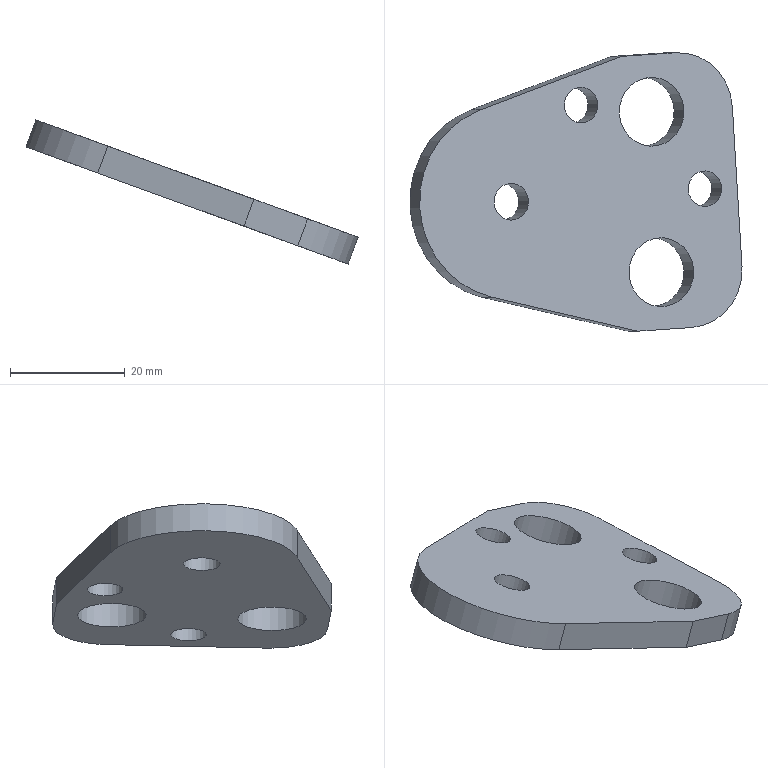Part | NX | features solid 2 | 1 solid | 15 faces | box 57.932 x 48.562 x 25.162 mm | volume 9858 mm3 | cylinder 8 | plane 7 | commonest cylinder face diameters 6.2 x2 12 x2 20 x2 6.4 x1 34 x1
STEP:
#1=CARTESIAN_POINT('',(737.004,494.915,31.011));
#2=VERTEX_POINT('',#1);
#3=CARTESIAN_POINT('',(746.983,485.575,27.379));
#4=VERTEX_POINT('',#3);
#5=CARTESIAN_POINT('',(737.605,484.935,30.792));
#6=DIRECTION('',(-0.342,0.,-0.9397));
#7=DIRECTION('',(0.9378,0.06398,-0.3413));
#8=AXIS2_PLACEMENT_3D('',#5,#6,#7);
#9=CIRCLE('',#8,10.);
#10=EDGE_CURVE('',#2,#4,#9,.T.);
#11=ORIENTED_EDGE('',*,*,#10,.F.);
#12=CARTESIAN_POINT('',(738.714,494.915,35.71));
#13=VERTEX_POINT('',#12);
#14=CARTESIAN_POINT('',(738.714,494.915,35.71));
#15=DIRECTION('',(-0.342,0.,-0.9397));
#16=VECTOR('',#15,1000.);
#17=LINE('',#14,#16);
#18=EDGE_CURVE('',#13,#2,#17,.T.);
#19=ORIENTED_EDGE('',*,*,#18,.F.);
#20=CARTESIAN_POINT('',(748.693,485.575,32.078));
#21=VERTEX_POINT('',#20);
#22=CARTESIAN_POINT('',(739.315,484.935,35.491));
#23=DIRECTION('',(-0.342,0.,-0.9397));
#24=DIRECTION('',(0.9378,0.06398,-0.3413));
#25=AXIS2_PLACEMENT_3D('',#22,#23,#24);
#26=CIRCLE('',#25,10.);
#27=EDGE_CURVE('',#13,#21,#26,.T.);
#28=ORIENTED_EDGE('',*,*,#27,.T.);
#29=CARTESIAN_POINT('',(748.693,485.575,32.078));
#30=DIRECTION('',(-0.342,0.,-0.9397));
#31=VECTOR('',#30,1000.);
#32=LINE('',#29,#31);
#33=EDGE_CURVE('',#21,#4,#32,.T.);
#34=ORIENTED_EDGE('',*,*,#33,.T.);
#35=EDGE_LOOP('',(#11,#19,#28,#34));
#36=FACE_BOUND('',#35,.T.);
#37=CARTESIAN_POINT('',(739.315,484.935,35.491));
#38=DIRECTION('',(-0.342,0.,-0.9397));
#39=DIRECTION('',(0.9378,0.06398,-0.3413));
#40=AXIS2_PLACEMENT_3D('',#37,#38,#39);
#41=CYLINDRICAL_SURFACE('',#40,10.);
#42=ADVANCED_FACE('',(#36),#41,.T.);
#43=CARTESIAN_POINT('',(748.666,457.633,26.766));
#44=VERTEX_POINT('',#43);
#45=CARTESIAN_POINT('',(748.666,457.633,26.766));
#46=DIRECTION('',(-0.06013,0.998,0.02188));
#47=VECTOR('',#46,1000.);
#48=LINE('',#45,#47);
#49=EDGE_CURVE('',#44,#4,#48,.T.);
#50=ORIENTED_EDGE('',*,*,#49,.T.);
#51=ORIENTED_EDGE('',*,*,#33,.F.);
#52=CARTESIAN_POINT('',(750.376,457.633,31.465));
#53=VERTEX_POINT('',#52);
#54=CARTESIAN_POINT('',(750.376,457.633,31.465));
#55=DIRECTION('',(-0.06013,0.998,0.02188));
#56=VECTOR('',#55,1000.);
#57=LINE('',#54,#56);
#58=EDGE_CURVE('',#53,#21,#57,.T.);
#59=ORIENTED_EDGE('',*,*,#58,.F.);
#60=CARTESIAN_POINT('',(750.376,457.633,31.465));
#61=DIRECTION('',(-0.342,0.,-0.9397));
#62=VECTOR('',#61,1000.);
#63=LINE('',#60,#62);
#64=EDGE_CURVE('',#53,#44,#63,.T.);
#65=ORIENTED_EDGE('',*,*,#64,.T.);
#66=EDGE_LOOP('',(#50,#51,#59,#65));
#67=FACE_BOUND('',#66,.T.);
#68=CARTESIAN_POINT('',(750.376,457.633,31.465));
#69=DIRECTION('',(-0.9378,-0.06398,0.3413));
#70=DIRECTION('',(0.06013,-0.998,-0.02188));
#71=AXIS2_PLACEMENT_3D('',#68,#69,#70);
#72=PLANE('',#71);
#73=ADVANCED_FACE('',(#67),#72,.F.);
#74=CARTESIAN_POINT('',(739.89,447.013,29.961));
#75=VERTEX_POINT('',#74);
#76=CARTESIAN_POINT('',(739.289,456.993,30.18));
#77=DIRECTION('',(-0.342,0.,-0.9397));
#78=DIRECTION('',(0.9378,0.06398,-0.3413));
#79=AXIS2_PLACEMENT_3D('',#76,#77,#78);
#80=CIRCLE('',#79,10.);
#81=EDGE_CURVE('',#44,#75,#80,.T.);
#82=ORIENTED_EDGE('',*,*,#81,.F.);
#83=ORIENTED_EDGE('',*,*,#64,.F.);
#84=CARTESIAN_POINT('',(741.6,447.013,34.659));
#85=VERTEX_POINT('',#84);
#86=CARTESIAN_POINT('',(740.999,456.993,34.878));
#87=DIRECTION('',(-0.342,0.,-0.9397));
#88=DIRECTION('',(0.9378,0.06398,-0.3413));
#89=AXIS2_PLACEMENT_3D('',#86,#87,#88);
#90=CIRCLE('',#89,10.);
#91=EDGE_CURVE('',#53,#85,#90,.T.);
#92=ORIENTED_EDGE('',*,*,#91,.T.);
#93=CARTESIAN_POINT('',(741.6,447.013,34.659));
#94=DIRECTION('',(-0.342,0.,-0.9397));
#95=VECTOR('',#94,1000.);
#96=LINE('',#93,#95);
#97=EDGE_CURVE('',#85,#75,#96,.T.);
#98=ORIENTED_EDGE('',*,*,#97,.T.);
#99=EDGE_LOOP('',(#82,#83,#92,#98));
#100=FACE_BOUND('',#99,.T.);
#101=CARTESIAN_POINT('',(740.999,456.993,34.878));
#102=DIRECTION('',(-0.342,0.,-0.9397));
#103=DIRECTION('',(0.9378,0.06398,-0.3413));
#104=AXIS2_PLACEMENT_3D('',#101,#102,#103);
#105=CYLINDRICAL_SURFACE('',#104,10.);
#106=ADVANCED_FACE('',(#100),#105,.T.);
#107=CARTESIAN_POINT('',(730.512,446.373,33.374));
#108=VERTEX_POINT('',#107);
#109=CARTESIAN_POINT('',(730.512,446.373,33.374));
#110=DIRECTION('',(0.9378,0.06398,-0.3413));
#111=VECTOR('',#110,1000.);
#112=LINE('',#109,#111);
#113=EDGE_CURVE('',#108,#75,#112,.T.);
#114=ORIENTED_EDGE('',*,*,#113,.T.);
#115=ORIENTED_EDGE('',*,*,#97,.F.);
#116=CARTESIAN_POINT('',(732.222,446.373,38.072));
#117=VERTEX_POINT('',#116);
#118=CARTESIAN_POINT('',(732.222,446.373,38.072));
#119=DIRECTION('',(0.9378,0.06398,-0.3413));
#120=VECTOR('',#119,1000.);
#121=LINE('',#118,#120);
#122=EDGE_CURVE('',#117,#85,#121,.T.);
#123=ORIENTED_EDGE('',*,*,#122,.F.);
#124=CARTESIAN_POINT('',(732.222,446.373,38.072));
#125=DIRECTION('',(-0.342,0.,-0.9397));
#126=VECTOR('',#125,1000.);
#127=LINE('',#124,#126);
#128=EDGE_CURVE('',#117,#108,#127,.T.);
#129=ORIENTED_EDGE('',*,*,#128,.T.);
#130=EDGE_LOOP('',(#114,#115,#123,#129));
#131=FACE_BOUND('',#130,.T.);
#132=CARTESIAN_POINT('',(732.222,446.373,38.072));
#133=DIRECTION('',(-0.06013,0.998,0.02188));
#134=DIRECTION('',(-0.9378,-0.06398,0.3413));
#135=AXIS2_PLACEMENT_3D('',#132,#133,#134);
#136=PLANE('',#135);
#137=ADVANCED_FACE('',(#131),#136,.F.);
#138=CARTESIAN_POINT('',(705.023,452.31,42.651));
#139=VERTEX_POINT('',#138);
#140=CARTESIAN_POINT('',(705.023,452.31,42.651));
#141=DIRECTION('',(0.918,-0.2138,-0.3341));
#142=VECTOR('',#141,1000.);
#143=LINE('',#140,#142);
#144=EDGE_CURVE('',#139,#108,#143,.T.);
#145=ORIENTED_EDGE('',*,*,#144,.T.);
#146=ORIENTED_EDGE('',*,*,#128,.F.);
#147=CARTESIAN_POINT('',(706.733,452.31,47.35));
#148=VERTEX_POINT('',#147);
#149=CARTESIAN_POINT('',(706.733,452.31,47.35));
#150=DIRECTION('',(0.918,-0.2138,-0.3341));
#151=VECTOR('',#150,1000.);
#152=LINE('',#149,#151);
#153=EDGE_CURVE('',#148,#117,#152,.T.);
#154=ORIENTED_EDGE('',*,*,#153,.F.);
#155=CARTESIAN_POINT('',(706.733,452.31,47.35));
#156=DIRECTION('',(-0.342,0.,-0.9397));
#157=VECTOR('',#156,1000.);
#158=LINE('',#155,#157);
#159=EDGE_CURVE('',#148,#139,#158,.T.);
#160=ORIENTED_EDGE('',*,*,#159,.T.);
#161=EDGE_LOOP('',(#145,#146,#154,#160));
#162=FACE_BOUND('',#161,.T.);
#163=CARTESIAN_POINT('',(706.733,452.31,47.35));
#164=DIRECTION('',(0.2009,0.9769,-0.07312));
#165=DIRECTION('',(-0.918,0.2138,0.3341));
#166=AXIS2_PLACEMENT_3D('',#163,#164,#165);
#167=PLANE('',#166);
#168=ADVANCED_FACE('',(#162),#167,.F.);
#169=CARTESIAN_POINT('',(703.058,484.924,43.366));
#170=VERTEX_POINT('',#169);
#171=CARTESIAN_POINT('',(708.438,468.917,41.408));
#172=DIRECTION('',(-0.342,0.,-0.9397));
#173=DIRECTION('',(0.9378,0.06398,-0.3413));
#174=AXIS2_PLACEMENT_3D('',#171,#172,#173);
#175=CIRCLE('',#174,17.);
#176=EDGE_CURVE('',#139,#170,#175,.T.);
#177=ORIENTED_EDGE('',*,*,#176,.F.);
#178=ORIENTED_EDGE('',*,*,#159,.F.);
#179=CARTESIAN_POINT('',(704.768,484.924,48.065));
#180=VERTEX_POINT('',#179);
#181=CARTESIAN_POINT('',(710.148,468.917,46.107));
#182=DIRECTION('',(-0.342,0.,-0.9397));
#183=DIRECTION('',(0.9378,0.06398,-0.3413));
#184=AXIS2_PLACEMENT_3D('',#181,#182,#183);
#185=CIRCLE('',#184,17.);
#186=EDGE_CURVE('',#148,#180,#185,.T.);
#187=ORIENTED_EDGE('',*,*,#186,.T.);
#188=CARTESIAN_POINT('',(704.768,484.924,48.065));
#189=DIRECTION('',(-0.342,0.,-0.9397));
#190=VECTOR('',#189,1000.);
#191=LINE('',#188,#190);
#192=EDGE_CURVE('',#180,#170,#191,.T.);
#193=ORIENTED_EDGE('',*,*,#192,.T.);
#194=EDGE_LOOP('',(#177,#178,#187,#193));
#195=FACE_BOUND('',#194,.T.);
#196=CARTESIAN_POINT('',(710.148,468.917,46.107));
#197=DIRECTION('',(-0.342,0.,-0.9397));
#198=DIRECTION('',(0.9378,0.06398,-0.3413));
#199=AXIS2_PLACEMENT_3D('',#196,#197,#198);
#200=CYLINDRICAL_SURFACE('',#199,17.);
#201=ADVANCED_FACE('',(#195),#200,.T.);
#202=CARTESIAN_POINT('',(727.626,494.275,34.424));
#203=VERTEX_POINT('',#202);
#204=CARTESIAN_POINT('',(703.058,484.924,43.366));
#205=DIRECTION('',(0.8848,0.3368,-0.322));
#206=VECTOR('',#205,1000.);
#207=LINE('',#204,#206);
#208=EDGE_CURVE('',#170,#203,#207,.T.);
#209=ORIENTED_EDGE('',*,*,#208,.F.);
#210=ORIENTED_EDGE('',*,*,#192,.F.);
#211=CARTESIAN_POINT('',(729.336,494.275,39.123));
#212=VERTEX_POINT('',#211);
#213=CARTESIAN_POINT('',(704.768,484.924,48.065));
#214=DIRECTION('',(0.8848,0.3368,-0.322));
#215=VECTOR('',#214,1000.);
#216=LINE('',#213,#215);
#217=EDGE_CURVE('',#180,#212,#216,.T.);
#218=ORIENTED_EDGE('',*,*,#217,.T.);
#219=CARTESIAN_POINT('',(729.336,494.275,39.123));
#220=DIRECTION('',(-0.342,0.,-0.9397));
#221=VECTOR('',#220,1000.);
#222=LINE('',#219,#221);
#223=EDGE_CURVE('',#212,#203,#222,.T.);
#224=ORIENTED_EDGE('',*,*,#223,.T.);
#225=EDGE_LOOP('',(#209,#210,#218,#224));
#226=FACE_BOUND('',#225,.T.);
#227=CARTESIAN_POINT('',(704.768,484.924,48.065));
#228=DIRECTION('',(-0.3165,0.9416,0.1152));
#229=DIRECTION('',(-0.8848,-0.3368,0.322));
#230=AXIS2_PLACEMENT_3D('',#227,#228,#229);
#231=PLANE('',#230);
#232=ADVANCED_FACE('',(#226),#231,.T.);
#233=CARTESIAN_POINT('',(727.626,494.275,34.424));
#234=DIRECTION('',(0.9378,0.06398,-0.3413));
#235=VECTOR('',#234,1000.);
#236=LINE('',#233,#235);
#237=EDGE_CURVE('',#203,#2,#236,.T.);
#238=ORIENTED_EDGE('',*,*,#237,.F.);
#239=ORIENTED_EDGE('',*,*,#223,.F.);
#240=CARTESIAN_POINT('',(729.336,494.275,39.123));
#241=DIRECTION('',(0.9378,0.06398,-0.3413));
#242=VECTOR('',#241,1000.);
#243=LINE('',#240,#242);
#244=EDGE_CURVE('',#212,#13,#243,.T.);
#245=ORIENTED_EDGE('',*,*,#244,.T.);
#246=ORIENTED_EDGE('',*,*,#18,.T.);
#247=EDGE_LOOP('',(#238,#239,#245,#246));
#248=FACE_BOUND('',#247,.T.);
#249=CARTESIAN_POINT('',(729.336,494.275,39.123));
#250=DIRECTION('',(-0.06013,0.998,0.02188));
#251=DIRECTION('',(-0.342,0.,-0.9397));
#252=AXIS2_PLACEMENT_3D('',#249,#250,#251);
#253=PLANE('',#252);
#254=ADVANCED_FACE('',(#248),#253,.T.);
#255=CARTESIAN_POINT('',(741.936,457.057,34.537));
#256=VERTEX_POINT('',#255);
#257=CARTESIAN_POINT('',(736.31,456.673,36.585));
#258=DIRECTION('',(-0.342,0.,-0.9397));
#259=DIRECTION('',(0.9378,0.06398,-0.3413));
#260=AXIS2_PLACEMENT_3D('',#257,#258,#259);
#261=CIRCLE('',#260,6.);
#262=EDGE_CURVE('',#256,#256,#261,.T.);
#263=ORIENTED_EDGE('',*,*,#262,.T.);
#264=EDGE_LOOP('',(#263));
#265=FACE_BOUND('',#264,.T.);
#266=CARTESIAN_POINT('',(740.253,484.999,35.149));
#267=VERTEX_POINT('',#266);
#268=CARTESIAN_POINT('',(734.626,484.616,37.197));
#269=DIRECTION('',(-0.342,0.,-0.9397));
#270=DIRECTION('',(0.9378,0.06398,-0.3413));
#271=AXIS2_PLACEMENT_3D('',#268,#269,#270);
#272=CIRCLE('',#271,6.);
#273=EDGE_CURVE('',#267,#267,#272,.T.);
#274=ORIENTED_EDGE('',*,*,#273,.T.);
#275=EDGE_LOOP('',(#274));
#276=FACE_BOUND('',#275,.T.);
#277=CARTESIAN_POINT('',(713.149,469.121,45.014));
#278=VERTEX_POINT('',#277);
#279=CARTESIAN_POINT('',(710.148,468.917,46.107));
#280=DIRECTION('',(-0.342,0.,-0.9397));
#281=DIRECTION('',(0.9378,0.06398,-0.3413));
#282=AXIS2_PLACEMENT_3D('',#279,#280,#281);
#283=CIRCLE('',#282,3.2);
#284=EDGE_CURVE('',#278,#278,#283,.T.);
#285=ORIENTED_EDGE('',*,*,#284,.T.);
#286=EDGE_LOOP('',(#285));
#287=FACE_BOUND('',#286,.T.);
#288=CARTESIAN_POINT('',(725.222,485.978,40.62));
#289=VERTEX_POINT('',#288);
#290=CARTESIAN_POINT('',(722.315,485.78,41.678));
#291=DIRECTION('',(-0.342,0.,-0.9397));
#292=DIRECTION('',(0.9378,0.06398,-0.3413));
#293=AXIS2_PLACEMENT_3D('',#290,#291,#292);
#294=CIRCLE('',#293,3.1);
#295=EDGE_CURVE('',#289,#289,#294,.T.);
#296=ORIENTED_EDGE('',*,*,#295,.T.);
#297=EDGE_LOOP('',(#296));
#298=FACE_BOUND('',#297,.T.);
#299=CARTESIAN_POINT('',(746.815,471.418,32.761));
#300=VERTEX_POINT('',#299);
#301=CARTESIAN_POINT('',(743.908,471.22,33.819));
#302=DIRECTION('',(-0.342,0.,-0.9397));
#303=DIRECTION('',(0.9378,0.06398,-0.3413));
#304=AXIS2_PLACEMENT_3D('',#301,#302,#303);
#305=CIRCLE('',#304,3.1);
#306=EDGE_CURVE('',#300,#300,#305,.T.);
#307=ORIENTED_EDGE('',*,*,#306,.T.);
#308=EDGE_LOOP('',(#307));
#309=FACE_BOUND('',#308,.T.);
#310=ORIENTED_EDGE('',*,*,#27,.F.);
#311=ORIENTED_EDGE('',*,*,#244,.F.);
#312=ORIENTED_EDGE('',*,*,#217,.F.);
#313=ORIENTED_EDGE('',*,*,#186,.F.);
#314=ORIENTED_EDGE('',*,*,#153,.T.);
#315=ORIENTED_EDGE('',*,*,#122,.T.);
#316=ORIENTED_EDGE('',*,*,#91,.F.);
#317=ORIENTED_EDGE('',*,*,#58,.T.);
#318=EDGE_LOOP('',(#310,#311,#312,#313,#314,#315,#316,#317));
#319=FACE_BOUND('',#318,.T.);
#320=CARTESIAN_POINT('',(739.315,484.935,35.491));
#321=DIRECTION('',(-0.342,0.,-0.9397));
#322=DIRECTION('',(0.9378,0.06398,-0.3413));
#323=AXIS2_PLACEMENT_3D('',#320,#321,#322);
#324=PLANE('',#323);
#325=ADVANCED_FACE('',(#265,#276,#287,#298,#309,#319),#324,.F.);
#326=CARTESIAN_POINT('',(740.226,457.057,29.838));
#327=VERTEX_POINT('',#326);
#328=CARTESIAN_POINT('',(734.6,456.673,31.886));
#329=DIRECTION('',(-0.342,0.,-0.9397));
#330=DIRECTION('',(0.9378,0.06398,-0.3413));
#331=AXIS2_PLACEMENT_3D('',#328,#329,#330);
#332=CIRCLE('',#331,6.);
#333=EDGE_CURVE('',#327,#327,#332,.T.);
#334=ORIENTED_EDGE('',*,*,#333,.F.);
#335=EDGE_LOOP('',(#334));
#336=FACE_BOUND('',#335,.T.);
#337=CARTESIAN_POINT('',(738.543,484.999,30.451));
#338=VERTEX_POINT('',#337);
#339=CARTESIAN_POINT('',(732.916,484.616,32.499));
#340=DIRECTION('',(-0.342,0.,-0.9397));
#341=DIRECTION('',(0.9378,0.06398,-0.3413));
#342=AXIS2_PLACEMENT_3D('',#339,#340,#341);
#343=CIRCLE('',#342,6.);
#344=EDGE_CURVE('',#338,#338,#343,.T.);
#345=ORIENTED_EDGE('',*,*,#344,.F.);
#346=EDGE_LOOP('',(#345));
#347=FACE_BOUND('',#346,.T.);
#348=CARTESIAN_POINT('',(711.439,469.121,40.316));
#349=VERTEX_POINT('',#348);
#350=CARTESIAN_POINT('',(708.438,468.917,41.408));
#351=DIRECTION('',(-0.342,0.,-0.9397));
#352=DIRECTION('',(0.9378,0.06398,-0.3413));
#353=AXIS2_PLACEMENT_3D('',#350,#351,#352);
#354=CIRCLE('',#353,3.2);
#355=EDGE_CURVE('',#349,#349,#354,.T.);
#356=ORIENTED_EDGE('',*,*,#355,.F.);
#357=EDGE_LOOP('',(#356));
#358=FACE_BOUND('',#357,.T.);
#359=CARTESIAN_POINT('',(723.512,485.978,35.922));
#360=VERTEX_POINT('',#359);
#361=CARTESIAN_POINT('',(720.605,485.78,36.98));
#362=DIRECTION('',(-0.342,0.,-0.9397));
#363=DIRECTION('',(0.9378,0.06398,-0.3413));
#364=AXIS2_PLACEMENT_3D('',#361,#362,#363);
#365=CIRCLE('',#364,3.1);
#366=EDGE_CURVE('',#360,#360,#365,.T.);
#367=ORIENTED_EDGE('',*,*,#366,.F.);
#368=EDGE_LOOP('',(#367));
#369=FACE_BOUND('',#368,.T.);
#370=CARTESIAN_POINT('',(745.105,471.418,28.063));
#371=VERTEX_POINT('',#370);
#372=CARTESIAN_POINT('',(742.198,471.22,29.121));
#373=DIRECTION('',(-0.342,0.,-0.9397));
#374=DIRECTION('',(0.9378,0.06398,-0.3413));
#375=AXIS2_PLACEMENT_3D('',#372,#373,#374);
#376=CIRCLE('',#375,3.1);
#377=EDGE_CURVE('',#371,#371,#376,.T.);
#378=ORIENTED_EDGE('',*,*,#377,.F.);
#379=EDGE_LOOP('',(#378));
#380=FACE_BOUND('',#379,.T.);
#381=ORIENTED_EDGE('',*,*,#10,.T.);
#382=ORIENTED_EDGE('',*,*,#49,.F.);
#383=ORIENTED_EDGE('',*,*,#81,.T.);
#384=ORIENTED_EDGE('',*,*,#113,.F.);
#385=ORIENTED_EDGE('',*,*,#144,.F.);
#386=ORIENTED_EDGE('',*,*,#176,.T.);
#387=ORIENTED_EDGE('',*,*,#208,.T.);
#388=ORIENTED_EDGE('',*,*,#237,.T.);
#389=EDGE_LOOP('',(#381,#382,#383,#384,#385,#386,#387,#388));
#390=FACE_BOUND('',#389,.T.);
#391=CARTESIAN_POINT('',(737.605,484.935,30.792));
#392=DIRECTION('',(-0.342,0.,-0.9397));
#393=DIRECTION('',(0.9378,0.06398,-0.3413));
#394=AXIS2_PLACEMENT_3D('',#391,#392,#393);
#395=PLANE('',#394);
#396=ADVANCED_FACE('',(#336,#347,#358,#369,#380,#390),#395,.T.);
#397=ORIENTED_EDGE('',*,*,#377,.T.);
#398=EDGE_LOOP('',(#397));
#399=FACE_BOUND('',#398,.T.);
#400=ORIENTED_EDGE('',*,*,#306,.F.);
#401=EDGE_LOOP('',(#400));
#402=FACE_BOUND('',#401,.T.);
#403=CARTESIAN_POINT('',(743.908,471.22,33.819));
#404=DIRECTION('',(-0.342,0.,-0.9397));
#405=DIRECTION('',(0.9378,0.06398,-0.3413));
#406=AXIS2_PLACEMENT_3D('',#403,#404,#405);
#407=CYLINDRICAL_SURFACE('',#406,3.1);
#408=ADVANCED_FACE('',(#399,#402),#407,.F.);
#409=ORIENTED_EDGE('',*,*,#366,.T.);
#410=EDGE_LOOP('',(#409));
#411=FACE_BOUND('',#410,.T.);
#412=ORIENTED_EDGE('',*,*,#295,.F.);
#413=EDGE_LOOP('',(#412));
#414=FACE_BOUND('',#413,.T.);
#415=CARTESIAN_POINT('',(722.315,485.78,41.678));
#416=DIRECTION('',(-0.342,0.,-0.9397));
#417=DIRECTION('',(0.9378,0.06398,-0.3413));
#418=AXIS2_PLACEMENT_3D('',#415,#416,#417);
#419=CYLINDRICAL_SURFACE('',#418,3.1);
#420=ADVANCED_FACE('',(#411,#414),#419,.F.);
#421=ORIENTED_EDGE('',*,*,#355,.T.);
#422=EDGE_LOOP('',(#421));
#423=FACE_BOUND('',#422,.T.);
#424=ORIENTED_EDGE('',*,*,#284,.F.);
#425=EDGE_LOOP('',(#424));
#426=FACE_BOUND('',#425,.T.);
#427=CARTESIAN_POINT('',(710.148,468.917,46.107));
#428=DIRECTION('',(-0.342,0.,-0.9397));
#429=DIRECTION('',(0.9378,0.06398,-0.3413));
#430=AXIS2_PLACEMENT_3D('',#427,#428,#429);
#431=CYLINDRICAL_SURFACE('',#430,3.2);
#432=ADVANCED_FACE('',(#423,#426),#431,.F.);
#433=ORIENTED_EDGE('',*,*,#344,.T.);
#434=EDGE_LOOP('',(#433));
#435=FACE_BOUND('',#434,.T.);
#436=ORIENTED_EDGE('',*,*,#273,.F.);
#437=EDGE_LOOP('',(#436));
#438=FACE_BOUND('',#437,.T.);
#439=CARTESIAN_POINT('',(734.626,484.616,37.197));
#440=DIRECTION('',(-0.342,0.,-0.9397));
#441=DIRECTION('',(0.9378,0.06398,-0.3413));
#442=AXIS2_PLACEMENT_3D('',#439,#440,#441);
#443=CYLINDRICAL_SURFACE('',#442,6.);
#444=ADVANCED_FACE('',(#435,#438),#443,.F.);
#445=ORIENTED_EDGE('',*,*,#333,.T.);
#446=EDGE_LOOP('',(#445));
#447=FACE_BOUND('',#446,.T.);
#448=ORIENTED_EDGE('',*,*,#262,.F.);
#449=EDGE_LOOP('',(#448));
#450=FACE_BOUND('',#449,.T.);
#451=CARTESIAN_POINT('',(736.31,456.673,36.585));
#452=DIRECTION('',(-0.342,0.,-0.9397));
#453=DIRECTION('',(0.9378,0.06398,-0.3413));
#454=AXIS2_PLACEMENT_3D('',#451,#452,#453);
#455=CYLINDRICAL_SURFACE('',#454,6.);
#456=ADVANCED_FACE('',(#447,#450),#455,.F.);
#457=CLOSED_SHELL('',(#42,#73,#106,#137,#168,#201,#232,#254,#325,#396,#408,#420,#432,#444,#456));
#458=MANIFOLD_SOLID_BREP('',#457);
#459=(LENGTH_UNIT()NAMED_UNIT(*)SI_UNIT(.MILLI.,.METRE.));
#460=UNCERTAINTY_MEASURE_WITH_UNIT(LENGTH_MEASURE(0.00001),#459,'','');
#461=(NAMED_UNIT(*)PLANE_ANGLE_UNIT()SI_UNIT($,.RADIAN.));
#462=(NAMED_UNIT(*)SI_UNIT($,.STERADIAN.)SOLID_ANGLE_UNIT());
#463=(GEOMETRIC_REPRESENTATION_CONTEXT(3)GLOBAL_UNCERTAINTY_ASSIGNED_CONTEXT((#460))GLOBAL_UNIT_ASSIGNED_CONTEXT((#459,#461,#462))REPRESENTATION_CONTEXT('',''));
#464=ADVANCED_BREP_SHAPE_REPRESENTATION('',(#458),#463);